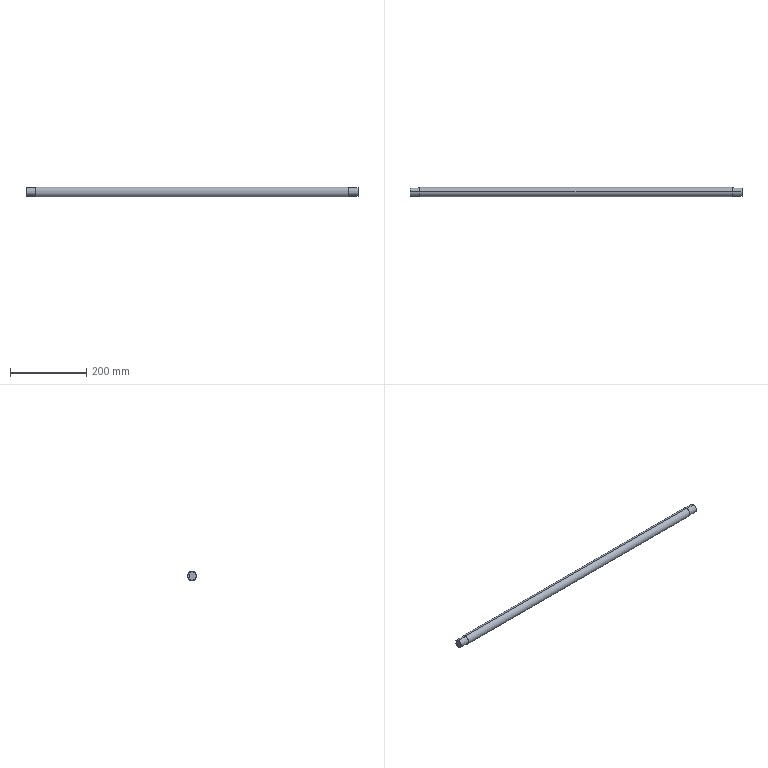Part | STEP file | Drive shaft | 1 solid | 18 faces | box 870 x 25 x 25 mm | volume 420131 mm3 | plane 10 | cylinder 8 | commonest cylinder face diameters 22 x4 8 x2 25 x2
STEP:
#1=CARTESIAN_POINT('',(410.,0.,12.5));
#2=VERTEX_POINT('',#1);
#3=CARTESIAN_POINT('',(410.,0.,-12.5));
#4=VERTEX_POINT('',#3);
#5=CARTESIAN_POINT('',(410.,0.,0.));
#6=DIRECTION('',(-1.,0.,0.));
#7=DIRECTION('',(0.,0.,1.));
#8=AXIS2_PLACEMENT_3D('',#5,#6,#7);
#9=CIRCLE('',#8,12.5);
#10=EDGE_CURVE('',#2,#4,#9,.T.);
#11=ORIENTED_EDGE('',*,*,#10,.T.);
#12=CARTESIAN_POINT('',(-410.,0.,-12.5));
#13=VERTEX_POINT('',#12);
#14=CARTESIAN_POINT('',(435.,0.,-12.5));
#15=DIRECTION('',(-1.,0.,0.));
#16=VECTOR('',#15,1000.);
#17=LINE('',#14,#16);
#18=EDGE_CURVE('',#4,#13,#17,.T.);
#19=ORIENTED_EDGE('',*,*,#18,.T.);
#20=CARTESIAN_POINT('',(-410.,0.,12.5));
#21=VERTEX_POINT('',#20);
#22=CARTESIAN_POINT('',(-410.,0.,0.));
#23=DIRECTION('',(1.,0.,0.));
#24=DIRECTION('',(0.,0.,1.));
#25=AXIS2_PLACEMENT_3D('',#22,#23,#24);
#26=CIRCLE('',#25,12.5);
#27=EDGE_CURVE('',#13,#21,#26,.T.);
#28=ORIENTED_EDGE('',*,*,#27,.T.);
#29=CARTESIAN_POINT('',(435.,0.,12.5));
#30=DIRECTION('',(-1.,0.,0.));
#31=VECTOR('',#30,1000.);
#32=LINE('',#29,#31);
#33=EDGE_CURVE('',#2,#21,#32,.T.);
#34=ORIENTED_EDGE('',*,*,#33,.F.);
#35=EDGE_LOOP('',(#11,#19,#28,#34));
#36=FACE_OUTER_BOUND('',#35,.T.);
#37=CARTESIAN_POINT('',(435.,0.,0.));
#38=DIRECTION('',(-1.,0.,0.));
#39=DIRECTION('',(0.,0.,1.));
#40=AXIS2_PLACEMENT_3D('',#37,#38,#39);
#41=CYLINDRICAL_SURFACE('',#40,12.5);
#42=ADVANCED_FACE('',(#36),#41,.T.);
#43=CARTESIAN_POINT('',(-410.,0.,-11.));
#44=VERTEX_POINT('',#43);
#45=CARTESIAN_POINT('',(-410.,0.,11.));
#46=VERTEX_POINT('',#45);
#47=CARTESIAN_POINT('',(-410.,0.,0.));
#48=DIRECTION('',(1.,0.,0.));
#49=DIRECTION('',(0.,0.,1.));
#50=AXIS2_PLACEMENT_3D('',#47,#48,#49);
#51=CIRCLE('',#50,11.);
#52=EDGE_CURVE('',#44,#46,#51,.T.);
#53=ORIENTED_EDGE('',*,*,#52,.F.);
#54=CARTESIAN_POINT('',(-435.,0.,-11.));
#55=VERTEX_POINT('',#54);
#56=CARTESIAN_POINT('',(-410.,0.,-11.));
#57=DIRECTION('',(-1.,0.,0.));
#58=VECTOR('',#57,1000.);
#59=LINE('',#56,#58);
#60=EDGE_CURVE('',#44,#55,#59,.T.);
#61=ORIENTED_EDGE('',*,*,#60,.T.);
#62=CARTESIAN_POINT('',(-435.,10.247,-4.));
#63=VERTEX_POINT('',#62);
#64=CARTESIAN_POINT('',(-435.,0.,0.));
#65=DIRECTION('',(1.,0.,0.));
#66=DIRECTION('',(0.,0.,1.));
#67=AXIS2_PLACEMENT_3D('',#64,#65,#66);
#68=CIRCLE('',#67,11.);
#69=EDGE_CURVE('',#55,#63,#68,.T.);
#70=ORIENTED_EDGE('',*,*,#69,.T.);
#71=CARTESIAN_POINT('',(-415.,10.247,-4.));
#72=VERTEX_POINT('',#71);
#73=CARTESIAN_POINT('',(-410.,10.247,-4.));
#74=DIRECTION('',(1.,0.,0.));
#75=VECTOR('',#74,1000.);
#76=LINE('',#73,#75);
#77=EDGE_CURVE('',#63,#72,#76,.T.);
#78=ORIENTED_EDGE('',*,*,#77,.T.);
#79=CARTESIAN_POINT('',(-415.,10.247,4.));
#80=VERTEX_POINT('',#79);
#81=CARTESIAN_POINT('',(-415.,10.247,-4.));
#82=CARTESIAN_POINT('',(-414.733,10.247,-4.));
#83=CARTESIAN_POINT('',(-414.472,10.257,-3.974));
#84=CARTESIAN_POINT('',(-413.958,10.297,-3.871));
#85=CARTESIAN_POINT('',(-413.702,10.326,-3.793));
#86=CARTESIAN_POINT('',(-413.219,10.398,-3.591));
#87=CARTESIAN_POINT('',(-412.991,10.44,-3.469));
#88=CARTESIAN_POINT('',(-412.558,10.532,-3.179));
#89=CARTESIAN_POINT('',(-412.355,10.581,-3.012));
#90=CARTESIAN_POINT('',(-411.989,10.679,-2.646));
#91=CARTESIAN_POINT('',(-411.824,10.727,-2.446));
#92=CARTESIAN_POINT('',(-411.532,10.817,-2.01));
#93=CARTESIAN_POINT('',(-411.409,10.858,-1.781));
#94=CARTESIAN_POINT('',(-411.208,10.926,-1.301));
#95=CARTESIAN_POINT('',(-411.13,10.953,-1.046));
#96=CARTESIAN_POINT('',(-411.026,10.99,-0.5291));
#97=CARTESIAN_POINT('',(-411.,11.,-0.268));
#98=CARTESIAN_POINT('',(-411.,11.,0.2589));
#99=CARTESIAN_POINT('',(-411.026,10.99,0.5264));
#100=CARTESIAN_POINT('',(-411.129,10.954,1.041));
#101=CARTESIAN_POINT('',(-411.205,10.927,1.292));
#102=CARTESIAN_POINT('',(-411.408,10.858,1.78));
#103=CARTESIAN_POINT('',(-411.532,10.817,2.01));
#104=CARTESIAN_POINT('',(-411.82,10.728,2.441));
#105=CARTESIAN_POINT('',(-411.988,10.679,2.644));
#106=CARTESIAN_POINT('',(-412.355,10.581,3.012));
#107=CARTESIAN_POINT('',(-412.554,10.533,3.176));
#108=CARTESIAN_POINT('',(-412.986,10.441,3.465));
#109=CARTESIAN_POINT('',(-413.219,10.398,3.591));
#110=CARTESIAN_POINT('',(-413.699,10.326,3.792));
#111=CARTESIAN_POINT('',(-413.949,10.297,3.868));
#112=CARTESIAN_POINT('',(-414.467,10.258,3.973));
#113=CARTESIAN_POINT('',(-414.733,10.247,4.));
#114=CARTESIAN_POINT('',(-415.,10.247,4.));
#115=B_SPLINE_CURVE_WITH_KNOTS('',3,(#81,#82,#83,#84,#85,#86,#87,#88,#89,#90,#91,#92,#93,#94,#95,#96,#97,#98,#99,#100,#101,#102,#103,#104,#105,#106,#107,#108,#109,#110,#111,#112,#113,#114),.UNSPECIFIED.,.F.,.F.,(4,2,2,2,2,2,2,2,2,2,2,2,2,2,2,2,4),(0.,0.0007881,0.001576,0.002364,0.003152,0.00394,0.004728,0.005517,0.006305,0.007093,0.007881,0.008669,0.009457,0.01025,0.01103,0.01182,0.01261),.UNSPECIFIED.);
#116=EDGE_CURVE('',#72,#80,#115,.T.);
#117=ORIENTED_EDGE('',*,*,#116,.T.);
#118=CARTESIAN_POINT('',(-435.,10.247,4.));
#119=VERTEX_POINT('',#118);
#120=CARTESIAN_POINT('',(-410.,10.247,4.));
#121=DIRECTION('',(-1.,0.,0.));
#122=VECTOR('',#121,1000.);
#123=LINE('',#120,#122);
#124=EDGE_CURVE('',#80,#119,#123,.T.);
#125=ORIENTED_EDGE('',*,*,#124,.T.);
#126=CARTESIAN_POINT('',(-435.,0.,11.));
#127=VERTEX_POINT('',#126);
#128=CARTESIAN_POINT('',(-435.,0.,0.));
#129=DIRECTION('',(1.,0.,0.));
#130=DIRECTION('',(0.,0.,1.));
#131=AXIS2_PLACEMENT_3D('',#128,#129,#130);
#132=CIRCLE('',#131,11.);
#133=EDGE_CURVE('',#119,#127,#132,.T.);
#134=ORIENTED_EDGE('',*,*,#133,.T.);
#135=CARTESIAN_POINT('',(-410.,0.,11.));
#136=DIRECTION('',(-1.,0.,0.));
#137=VECTOR('',#136,1000.);
#138=LINE('',#135,#137);
#139=EDGE_CURVE('',#46,#127,#138,.T.);
#140=ORIENTED_EDGE('',*,*,#139,.F.);
#141=EDGE_LOOP('',(#53,#61,#70,#78,#117,#125,#134,#140));
#142=FACE_OUTER_BOUND('',#141,.T.);
#143=CARTESIAN_POINT('',(-410.,0.,0.));
#144=DIRECTION('',(-1.,0.,0.));
#145=DIRECTION('',(0.,0.,1.));
#146=AXIS2_PLACEMENT_3D('',#143,#144,#145);
#147=CYLINDRICAL_SURFACE('',#146,11.);
#148=ADVANCED_FACE('',(#142),#147,.T.);
#149=CARTESIAN_POINT('',(410.,0.,11.));
#150=VERTEX_POINT('',#149);
#151=CARTESIAN_POINT('',(410.,0.,-11.));
#152=VERTEX_POINT('',#151);
#153=CARTESIAN_POINT('',(410.,0.,0.));
#154=DIRECTION('',(-1.,0.,0.));
#155=DIRECTION('',(0.,0.,-1.));
#156=AXIS2_PLACEMENT_3D('',#153,#154,#155);
#157=CIRCLE('',#156,11.);
#158=EDGE_CURVE('',#150,#152,#157,.T.);
#159=ORIENTED_EDGE('',*,*,#158,.F.);
#160=CARTESIAN_POINT('',(435.,0.,11.));
#161=VERTEX_POINT('',#160);
#162=CARTESIAN_POINT('',(410.,0.,11.));
#163=DIRECTION('',(1.,0.,0.));
#164=VECTOR('',#163,1000.);
#165=LINE('',#162,#164);
#166=EDGE_CURVE('',#150,#161,#165,.T.);
#167=ORIENTED_EDGE('',*,*,#166,.T.);
#168=CARTESIAN_POINT('',(435.,10.247,4.));
#169=VERTEX_POINT('',#168);
#170=CARTESIAN_POINT('',(435.,0.,0.));
#171=DIRECTION('',(-1.,0.,0.));
#172=DIRECTION('',(0.,0.,-1.));
#173=AXIS2_PLACEMENT_3D('',#170,#171,#172);
#174=CIRCLE('',#173,11.);
#175=EDGE_CURVE('',#161,#169,#174,.T.);
#176=ORIENTED_EDGE('',*,*,#175,.T.);
#177=CARTESIAN_POINT('',(415.,10.247,4.));
#178=VERTEX_POINT('',#177);
#179=CARTESIAN_POINT('',(410.,10.247,4.));
#180=DIRECTION('',(-1.,0.,0.));
#181=VECTOR('',#180,1000.);
#182=LINE('',#179,#181);
#183=EDGE_CURVE('',#169,#178,#182,.T.);
#184=ORIENTED_EDGE('',*,*,#183,.T.);
#185=CARTESIAN_POINT('',(415.,10.247,-4.));
#186=VERTEX_POINT('',#185);
#187=CARTESIAN_POINT('',(415.,10.247,4.));
#188=CARTESIAN_POINT('',(414.733,10.247,4.));
#189=CARTESIAN_POINT('',(414.472,10.257,3.974));
#190=CARTESIAN_POINT('',(413.958,10.297,3.871));
#191=CARTESIAN_POINT('',(413.702,10.326,3.793));
#192=CARTESIAN_POINT('',(413.219,10.398,3.591));
#193=CARTESIAN_POINT('',(412.991,10.44,3.469));
#194=CARTESIAN_POINT('',(412.558,10.532,3.179));
#195=CARTESIAN_POINT('',(412.355,10.581,3.012));
#196=CARTESIAN_POINT('',(411.989,10.679,2.646));
#197=CARTESIAN_POINT('',(411.824,10.727,2.446));
#198=CARTESIAN_POINT('',(411.532,10.817,2.01));
#199=CARTESIAN_POINT('',(411.409,10.858,1.781));
#200=CARTESIAN_POINT('',(411.208,10.926,1.301));
#201=CARTESIAN_POINT('',(411.13,10.953,1.046));
#202=CARTESIAN_POINT('',(411.026,10.99,0.5291));
#203=CARTESIAN_POINT('',(411.,11.,0.268));
#204=CARTESIAN_POINT('',(411.,11.,-0.2589));
#205=CARTESIAN_POINT('',(411.026,10.99,-0.5264));
#206=CARTESIAN_POINT('',(411.129,10.954,-1.041));
#207=CARTESIAN_POINT('',(411.205,10.927,-1.292));
#208=CARTESIAN_POINT('',(411.408,10.858,-1.78));
#209=CARTESIAN_POINT('',(411.532,10.817,-2.01));
#210=CARTESIAN_POINT('',(411.82,10.728,-2.441));
#211=CARTESIAN_POINT('',(411.988,10.679,-2.644));
#212=CARTESIAN_POINT('',(412.355,10.581,-3.012));
#213=CARTESIAN_POINT('',(412.554,10.533,-3.176));
#214=CARTESIAN_POINT('',(412.986,10.441,-3.465));
#215=CARTESIAN_POINT('',(413.219,10.398,-3.591));
#216=CARTESIAN_POINT('',(413.699,10.326,-3.792));
#217=CARTESIAN_POINT('',(413.949,10.297,-3.868));
#218=CARTESIAN_POINT('',(414.467,10.258,-3.973));
#219=CARTESIAN_POINT('',(414.733,10.247,-4.));
#220=CARTESIAN_POINT('',(415.,10.247,-4.));
#221=B_SPLINE_CURVE_WITH_KNOTS('',3,(#187,#188,#189,#190,#191,#192,#193,#194,#195,#196,#197,#198,#199,#200,#201,#202,#203,#204,#205,#206,#207,#208,#209,#210,#211,#212,#213,#214,#215,#216,#217,#218,#219,#220),.UNSPECIFIED.,.F.,.F.,(4,2,2,2,2,2,2,2,2,2,2,2,2,2,2,2,4),(0.,0.0007881,0.001576,0.002364,0.003152,0.00394,0.004728,0.005517,0.006305,0.007093,0.007881,0.008669,0.009457,0.01025,0.01103,0.01182,0.01261),.UNSPECIFIED.);
#222=EDGE_CURVE('',#178,#186,#221,.T.);
#223=ORIENTED_EDGE('',*,*,#222,.T.);
#224=CARTESIAN_POINT('',(435.,10.247,-4.));
#225=VERTEX_POINT('',#224);
#226=CARTESIAN_POINT('',(410.,10.247,-4.));
#227=DIRECTION('',(1.,0.,0.));
#228=VECTOR('',#227,1000.);
#229=LINE('',#226,#228);
#230=EDGE_CURVE('',#186,#225,#229,.T.);
#231=ORIENTED_EDGE('',*,*,#230,.T.);
#232=CARTESIAN_POINT('',(435.,0.,-11.));
#233=VERTEX_POINT('',#232);
#234=CARTESIAN_POINT('',(435.,0.,0.));
#235=DIRECTION('',(-1.,0.,0.));
#236=DIRECTION('',(0.,0.,-1.));
#237=AXIS2_PLACEMENT_3D('',#234,#235,#236);
#238=CIRCLE('',#237,11.);
#239=EDGE_CURVE('',#225,#233,#238,.T.);
#240=ORIENTED_EDGE('',*,*,#239,.T.);
#241=CARTESIAN_POINT('',(410.,0.,-11.));
#242=DIRECTION('',(1.,0.,0.));
#243=VECTOR('',#242,1000.);
#244=LINE('',#241,#243);
#245=EDGE_CURVE('',#152,#233,#244,.T.);
#246=ORIENTED_EDGE('',*,*,#245,.F.);
#247=EDGE_LOOP('',(#159,#167,#176,#184,#223,#231,#240,#246));
#248=FACE_OUTER_BOUND('',#247,.T.);
#249=CARTESIAN_POINT('',(410.,0.,0.));
#250=DIRECTION('',(1.,0.,0.));
#251=DIRECTION('',(0.,0.,-1.));
#252=AXIS2_PLACEMENT_3D('',#249,#250,#251);
#253=CYLINDRICAL_SURFACE('',#252,11.);
#254=ADVANCED_FACE('',(#248),#253,.T.);
#255=ORIENTED_EDGE('',*,*,#18,.F.);
#256=CARTESIAN_POINT('',(410.,0.,0.));
#257=DIRECTION('',(-1.,0.,0.));
#258=DIRECTION('',(0.,0.,1.));
#259=AXIS2_PLACEMENT_3D('',#256,#257,#258);
#260=CIRCLE('',#259,12.5);
#261=EDGE_CURVE('',#4,#2,#260,.T.);
#262=ORIENTED_EDGE('',*,*,#261,.T.);
#263=ORIENTED_EDGE('',*,*,#33,.T.);
#264=CARTESIAN_POINT('',(-410.,0.,0.));
#265=DIRECTION('',(1.,0.,0.));
#266=DIRECTION('',(0.,0.,1.));
#267=AXIS2_PLACEMENT_3D('',#264,#265,#266);
#268=CIRCLE('',#267,12.5);
#269=EDGE_CURVE('',#21,#13,#268,.T.);
#270=ORIENTED_EDGE('',*,*,#269,.T.);
#271=EDGE_LOOP('',(#255,#262,#263,#270));
#272=FACE_OUTER_BOUND('',#271,.T.);
#273=CARTESIAN_POINT('',(435.,0.,0.));
#274=DIRECTION('',(-1.,0.,0.));
#275=DIRECTION('',(0.,0.,1.));
#276=AXIS2_PLACEMENT_3D('',#273,#274,#275);
#277=CYLINDRICAL_SURFACE('',#276,12.5);
#278=ADVANCED_FACE('',(#272),#277,.T.);
#279=ORIENTED_EDGE('',*,*,#269,.F.);
#280=ORIENTED_EDGE('',*,*,#27,.F.);
#281=EDGE_LOOP('',(#279,#280));
#282=FACE_OUTER_BOUND('',#281,.T.);
#283=CARTESIAN_POINT('',(-410.,0.,0.));
#284=DIRECTION('',(1.,0.,0.));
#285=DIRECTION('',(0.,0.,1.));
#286=AXIS2_PLACEMENT_3D('',#283,#284,#285);
#287=CIRCLE('',#286,11.);
#288=EDGE_CURVE('',#46,#44,#287,.T.);
#289=ORIENTED_EDGE('',*,*,#288,.T.);
#290=ORIENTED_EDGE('',*,*,#52,.T.);
#291=EDGE_LOOP('',(#289,#290));
#292=FACE_BOUND('',#291,.T.);
#293=CARTESIAN_POINT('',(-410.,0.,0.));
#294=DIRECTION('',(-1.,0.,0.));
#295=DIRECTION('',(0.,0.,1.));
#296=AXIS2_PLACEMENT_3D('',#293,#294,#295);
#297=PLANE('',#296);
#298=ADVANCED_FACE('',(#282,#292),#297,.T.);
#299=ORIENTED_EDGE('',*,*,#10,.F.);
#300=ORIENTED_EDGE('',*,*,#261,.F.);
#301=EDGE_LOOP('',(#299,#300));
#302=FACE_OUTER_BOUND('',#301,.T.);
#303=CARTESIAN_POINT('',(410.,0.,0.));
#304=DIRECTION('',(-1.,0.,0.));
#305=DIRECTION('',(0.,0.,-1.));
#306=AXIS2_PLACEMENT_3D('',#303,#304,#305);
#307=CIRCLE('',#306,11.);
#308=EDGE_CURVE('',#152,#150,#307,.T.);
#309=ORIENTED_EDGE('',*,*,#308,.T.);
#310=ORIENTED_EDGE('',*,*,#158,.T.);
#311=EDGE_LOOP('',(#309,#310));
#312=FACE_BOUND('',#311,.T.);
#313=CARTESIAN_POINT('',(410.,0.,0.));
#314=DIRECTION('',(1.,0.,0.));
#315=DIRECTION('',(0.,0.,-1.));
#316=AXIS2_PLACEMENT_3D('',#313,#314,#315);
#317=PLANE('',#316);
#318=ADVANCED_FACE('',(#302,#312),#317,.T.);
#319=ORIENTED_EDGE('',*,*,#60,.F.);
#320=ORIENTED_EDGE('',*,*,#288,.F.);
#321=ORIENTED_EDGE('',*,*,#139,.T.);
#322=CARTESIAN_POINT('',(-435.,0.,0.));
#323=DIRECTION('',(1.,0.,0.));
#324=DIRECTION('',(0.,0.,1.));
#325=AXIS2_PLACEMENT_3D('',#322,#323,#324);
#326=CIRCLE('',#325,11.);
#327=EDGE_CURVE('',#127,#55,#326,.T.);
#328=ORIENTED_EDGE('',*,*,#327,.T.);
#329=EDGE_LOOP('',(#319,#320,#321,#328));
#330=FACE_OUTER_BOUND('',#329,.T.);
#331=CARTESIAN_POINT('',(-410.,0.,0.));
#332=DIRECTION('',(-1.,0.,0.));
#333=DIRECTION('',(0.,0.,1.));
#334=AXIS2_PLACEMENT_3D('',#331,#332,#333);
#335=CYLINDRICAL_SURFACE('',#334,11.);
#336=ADVANCED_FACE('',(#330),#335,.T.);
#337=ORIENTED_EDGE('',*,*,#166,.F.);
#338=ORIENTED_EDGE('',*,*,#308,.F.);
#339=ORIENTED_EDGE('',*,*,#245,.T.);
#340=CARTESIAN_POINT('',(435.,0.,0.));
#341=DIRECTION('',(-1.,0.,0.));
#342=DIRECTION('',(0.,0.,-1.));
#343=AXIS2_PLACEMENT_3D('',#340,#341,#342);
#344=CIRCLE('',#343,11.);
#345=EDGE_CURVE('',#233,#161,#344,.T.);
#346=ORIENTED_EDGE('',*,*,#345,.T.);
#347=EDGE_LOOP('',(#337,#338,#339,#346));
#348=FACE_OUTER_BOUND('',#347,.T.);
#349=CARTESIAN_POINT('',(410.,0.,0.));
#350=DIRECTION('',(1.,0.,0.));
#351=DIRECTION('',(0.,0.,-1.));
#352=AXIS2_PLACEMENT_3D('',#349,#350,#351);
#353=CYLINDRICAL_SURFACE('',#352,11.);
#354=ADVANCED_FACE('',(#348),#353,.T.);
#355=CARTESIAN_POINT('',(-435.,7.,-4.));
#356=VERTEX_POINT('',#355);
#357=CARTESIAN_POINT('',(-435.,0.,-4.));
#358=DIRECTION('',(0.,-1.,0.));
#359=VECTOR('',#358,1000.);
#360=LINE('',#357,#359);
#361=EDGE_CURVE('',#63,#356,#360,.T.);
#362=ORIENTED_EDGE('',*,*,#361,.F.);
#363=ORIENTED_EDGE('',*,*,#69,.F.);
#364=ORIENTED_EDGE('',*,*,#327,.F.);
#365=ORIENTED_EDGE('',*,*,#133,.F.);
#366=CARTESIAN_POINT('',(-435.,7.,4.));
#367=VERTEX_POINT('',#366);
#368=CARTESIAN_POINT('',(-435.,0.,4.));
#369=DIRECTION('',(0.,1.,0.));
#370=VECTOR('',#369,1000.);
#371=LINE('',#368,#370);
#372=EDGE_CURVE('',#367,#119,#371,.T.);
#373=ORIENTED_EDGE('',*,*,#372,.F.);
#374=CARTESIAN_POINT('',(-435.,7.,0.));
#375=DIRECTION('',(0.,0.,1.));
#376=VECTOR('',#375,1000.);
#377=LINE('',#374,#376);
#378=EDGE_CURVE('',#356,#367,#377,.T.);
#379=ORIENTED_EDGE('',*,*,#378,.F.);
#380=EDGE_LOOP('',(#362,#363,#364,#365,#373,#379));
#381=FACE_OUTER_BOUND('',#380,.T.);
#382=CARTESIAN_POINT('',(-435.,0.,0.));
#383=DIRECTION('',(1.,0.,0.));
#384=DIRECTION('',(0.,0.,-1.));
#385=AXIS2_PLACEMENT_3D('',#382,#383,#384);
#386=PLANE('',#385);
#387=ADVANCED_FACE('',(#381),#386,.F.);
#388=CARTESIAN_POINT('',(-415.,7.,4.));
#389=VERTEX_POINT('',#388);
#390=CARTESIAN_POINT('',(-415.,7.,4.));
#391=DIRECTION('',(1.,0.,0.));
#392=VECTOR('',#391,1000.);
#393=LINE('',#390,#392);
#394=EDGE_CURVE('',#367,#389,#393,.T.);
#395=ORIENTED_EDGE('',*,*,#394,.F.);
#396=ORIENTED_EDGE('',*,*,#372,.T.);
#397=ORIENTED_EDGE('',*,*,#124,.F.);
#398=CARTESIAN_POINT('',(-415.,12.5,4.));
#399=DIRECTION('',(0.,1.,0.));
#400=VECTOR('',#399,1000.);
#401=LINE('',#398,#400);
#402=EDGE_CURVE('',#389,#80,#401,.T.);
#403=ORIENTED_EDGE('',*,*,#402,.F.);
#404=EDGE_LOOP('',(#395,#396,#397,#403));
#405=FACE_OUTER_BOUND('',#404,.T.);
#406=CARTESIAN_POINT('',(-415.,12.5,4.));
#407=DIRECTION('',(0.,0.,1.));
#408=DIRECTION('',(1.,0.,0.));
#409=AXIS2_PLACEMENT_3D('',#406,#407,#408);
#410=PLANE('',#409);
#411=ADVANCED_FACE('',(#405),#410,.F.);
#412=CARTESIAN_POINT('',(-415.,7.,-4.));
#413=VERTEX_POINT('',#412);
#414=CARTESIAN_POINT('',(-415.,7.,0.));
#415=DIRECTION('',(0.,1.,0.));
#416=DIRECTION('',(0.,0.,-1.));
#417=AXIS2_PLACEMENT_3D('',#414,#415,#416);
#418=CIRCLE('',#417,4.);
#419=EDGE_CURVE('',#389,#413,#418,.T.);
#420=ORIENTED_EDGE('',*,*,#419,.F.);
#421=ORIENTED_EDGE('',*,*,#402,.T.);
#422=ORIENTED_EDGE('',*,*,#116,.F.);
#423=CARTESIAN_POINT('',(-415.,12.5,-4.));
#424=DIRECTION('',(0.,1.,0.));
#425=VECTOR('',#424,1000.);
#426=LINE('',#423,#425);
#427=EDGE_CURVE('',#413,#72,#426,.T.);
#428=ORIENTED_EDGE('',*,*,#427,.F.);
#429=EDGE_LOOP('',(#420,#421,#422,#428));
#430=FACE_OUTER_BOUND('',#429,.T.);
#431=CARTESIAN_POINT('',(-415.,12.5,0.));
#432=DIRECTION('',(0.,-1.,0.));
#433=DIRECTION('',(0.,0.,-1.));
#434=AXIS2_PLACEMENT_3D('',#431,#432,#433);
#435=CYLINDRICAL_SURFACE('',#434,4.);
#436=ADVANCED_FACE('',(#430),#435,.F.);
#437=CARTESIAN_POINT('',(-415.,7.,-4.));
#438=DIRECTION('',(-1.,0.,0.));
#439=VECTOR('',#438,1000.);
#440=LINE('',#437,#439);
#441=EDGE_CURVE('',#413,#356,#440,.T.);
#442=ORIENTED_EDGE('',*,*,#441,.F.);
#443=ORIENTED_EDGE('',*,*,#427,.T.);
#444=ORIENTED_EDGE('',*,*,#77,.F.);
#445=ORIENTED_EDGE('',*,*,#361,.T.);
#446=EDGE_LOOP('',(#442,#443,#444,#445));
#447=FACE_OUTER_BOUND('',#446,.T.);
#448=CARTESIAN_POINT('',(-415.,12.5,-4.));
#449=DIRECTION('',(0.,0.,-1.));
#450=DIRECTION('',(-1.,0.,0.));
#451=AXIS2_PLACEMENT_3D('',#448,#449,#450);
#452=PLANE('',#451);
#453=ADVANCED_FACE('',(#447),#452,.F.);
#454=ORIENTED_EDGE('',*,*,#239,.F.);
#455=CARTESIAN_POINT('',(435.,7.,-4.));
#456=VERTEX_POINT('',#455);
#457=CARTESIAN_POINT('',(435.,0.,-4.));
#458=DIRECTION('',(0.,-1.,0.));
#459=VECTOR('',#458,1000.);
#460=LINE('',#457,#459);
#461=EDGE_CURVE('',#225,#456,#460,.T.);
#462=ORIENTED_EDGE('',*,*,#461,.T.);
#463=CARTESIAN_POINT('',(435.,7.,4.));
#464=VERTEX_POINT('',#463);
#465=CARTESIAN_POINT('',(435.,7.,0.));
#466=DIRECTION('',(0.,0.,1.));
#467=VECTOR('',#466,1000.);
#468=LINE('',#465,#467);
#469=EDGE_CURVE('',#456,#464,#468,.T.);
#470=ORIENTED_EDGE('',*,*,#469,.T.);
#471=CARTESIAN_POINT('',(435.,0.,4.));
#472=DIRECTION('',(0.,1.,0.));
#473=VECTOR('',#472,1000.);
#474=LINE('',#471,#473);
#475=EDGE_CURVE('',#464,#169,#474,.T.);
#476=ORIENTED_EDGE('',*,*,#475,.T.);
#477=ORIENTED_EDGE('',*,*,#175,.F.);
#478=ORIENTED_EDGE('',*,*,#345,.F.);
#479=EDGE_LOOP('',(#454,#462,#470,#476,#477,#478));
#480=FACE_OUTER_BOUND('',#479,.T.);
#481=CARTESIAN_POINT('',(435.,0.,0.));
#482=DIRECTION('',(1.,0.,0.));
#483=DIRECTION('',(0.,0.,-1.));
#484=AXIS2_PLACEMENT_3D('',#481,#482,#483);
#485=PLANE('',#484);
#486=ADVANCED_FACE('',(#480),#485,.T.);
#487=ORIENTED_EDGE('',*,*,#461,.F.);
#488=ORIENTED_EDGE('',*,*,#230,.F.);
#489=CARTESIAN_POINT('',(415.,7.,-4.));
#490=VERTEX_POINT('',#489);
#491=CARTESIAN_POINT('',(415.,12.5,-4.));
#492=DIRECTION('',(0.,-1.,0.));
#493=VECTOR('',#492,1000.);
#494=LINE('',#491,#493);
#495=EDGE_CURVE('',#186,#490,#494,.T.);
#496=ORIENTED_EDGE('',*,*,#495,.T.);
#497=CARTESIAN_POINT('',(415.,7.,-4.));
#498=DIRECTION('',(1.,0.,0.));
#499=VECTOR('',#498,1000.);
#500=LINE('',#497,#499);
#501=EDGE_CURVE('',#490,#456,#500,.T.);
#502=ORIENTED_EDGE('',*,*,#501,.T.);
#503=EDGE_LOOP('',(#487,#488,#496,#502));
#504=FACE_OUTER_BOUND('',#503,.T.);
#505=CARTESIAN_POINT('',(415.,12.5,-4.));
#506=DIRECTION('',(0.,0.,1.));
#507=DIRECTION('',(1.,0.,0.));
#508=AXIS2_PLACEMENT_3D('',#505,#506,#507);
#509=PLANE('',#508);
#510=ADVANCED_FACE('',(#504),#509,.T.);
#511=CARTESIAN_POINT('',(415.,7.,4.));
#512=VERTEX_POINT('',#511);
#513=CARTESIAN_POINT('',(415.,7.,0.));
#514=DIRECTION('',(0.,1.,0.));
#515=DIRECTION('',(0.,0.,-1.));
#516=AXIS2_PLACEMENT_3D('',#513,#514,#515);
#517=CIRCLE('',#516,4.);
#518=EDGE_CURVE('',#490,#512,#517,.T.);
#519=ORIENTED_EDGE('',*,*,#518,.F.);
#520=ORIENTED_EDGE('',*,*,#495,.F.);
#521=ORIENTED_EDGE('',*,*,#222,.F.);
#522=CARTESIAN_POINT('',(415.,12.5,4.));
#523=DIRECTION('',(0.,1.,0.));
#524=VECTOR('',#523,1000.);
#525=LINE('',#522,#524);
#526=EDGE_CURVE('',#512,#178,#525,.T.);
#527=ORIENTED_EDGE('',*,*,#526,.F.);
#528=EDGE_LOOP('',(#519,#520,#521,#527));
#529=FACE_OUTER_BOUND('',#528,.T.);
#530=CARTESIAN_POINT('',(415.,12.5,0.));
#531=DIRECTION('',(0.,-1.,0.));
#532=DIRECTION('',(0.,0.,-1.));
#533=AXIS2_PLACEMENT_3D('',#530,#531,#532);
#534=CYLINDRICAL_SURFACE('',#533,4.);
#535=ADVANCED_FACE('',(#529),#534,.F.);
#536=ORIENTED_EDGE('',*,*,#526,.T.);
#537=ORIENTED_EDGE('',*,*,#183,.F.);
#538=ORIENTED_EDGE('',*,*,#475,.F.);
#539=CARTESIAN_POINT('',(415.,7.,4.));
#540=DIRECTION('',(-1.,0.,0.));
#541=VECTOR('',#540,1000.);
#542=LINE('',#539,#541);
#543=EDGE_CURVE('',#464,#512,#542,.T.);
#544=ORIENTED_EDGE('',*,*,#543,.T.);
#545=EDGE_LOOP('',(#536,#537,#538,#544));
#546=FACE_OUTER_BOUND('',#545,.T.);
#547=CARTESIAN_POINT('',(415.,12.5,4.));
#548=DIRECTION('',(0.,0.,-1.));
#549=DIRECTION('',(-1.,0.,0.));
#550=AXIS2_PLACEMENT_3D('',#547,#548,#549);
#551=PLANE('',#550);
#552=ADVANCED_FACE('',(#546),#551,.T.);
#553=ORIENTED_EDGE('',*,*,#419,.T.);
#554=ORIENTED_EDGE('',*,*,#441,.T.);
#555=ORIENTED_EDGE('',*,*,#378,.T.);
#556=ORIENTED_EDGE('',*,*,#394,.T.);
#557=EDGE_LOOP('',(#553,#554,#555,#556));
#558=FACE_OUTER_BOUND('',#557,.T.);
#559=CARTESIAN_POINT('',(-415.,7.,0.));
#560=DIRECTION('',(0.,1.,0.));
#561=DIRECTION('',(0.,0.,1.));
#562=AXIS2_PLACEMENT_3D('',#559,#560,#561);
#563=PLANE('',#562);
#564=ADVANCED_FACE('',(#558),#563,.T.);
#565=ORIENTED_EDGE('',*,*,#543,.F.);
#566=ORIENTED_EDGE('',*,*,#469,.F.);
#567=ORIENTED_EDGE('',*,*,#501,.F.);
#568=ORIENTED_EDGE('',*,*,#518,.T.);
#569=EDGE_LOOP('',(#565,#566,#567,#568));
#570=FACE_OUTER_BOUND('',#569,.T.);
#571=CARTESIAN_POINT('',(415.,7.,0.));
#572=DIRECTION('',(0.,1.,0.));
#573=DIRECTION('',(0.,0.,1.));
#574=AXIS2_PLACEMENT_3D('',#571,#572,#573);
#575=PLANE('',#574);
#576=ADVANCED_FACE('',(#570),#575,.T.);
#577=CLOSED_SHELL('',(#42,#148,#254,#278,#298,#318,#336,#354,#387,#411,#436,#453,#486,#510,#535,#552,#564,#576));
#578=MANIFOLD_SOLID_BREP('',#577);
#579=CARTESIAN_POINT('',(0.,0.,0.));
#580=DIRECTION('',(0.,0.,1.));
#581=DIRECTION('',(1.,0.,0.));
#582=AXIS2_PLACEMENT_3D('',#579,#580,#581);
#583=(LENGTH_UNIT()NAMED_UNIT(*)SI_UNIT(.MILLI.,.METRE.));
#584=UNCERTAINTY_MEASURE_WITH_UNIT(LENGTH_MEASURE(0.00001),#583,'','');
#585=(NAMED_UNIT(*)PLANE_ANGLE_UNIT()SI_UNIT($,.RADIAN.));
#586=(NAMED_UNIT(*)SI_UNIT($,.STERADIAN.)SOLID_ANGLE_UNIT());
#587=(GEOMETRIC_REPRESENTATION_CONTEXT(3)GLOBAL_UNCERTAINTY_ASSIGNED_CONTEXT((#584))GLOBAL_UNIT_ASSIGNED_CONTEXT((#583,#585,#586))REPRESENTATION_CONTEXT('',''));
#588=ADVANCED_BREP_SHAPE_REPRESENTATION('',(#578,#582),#587);